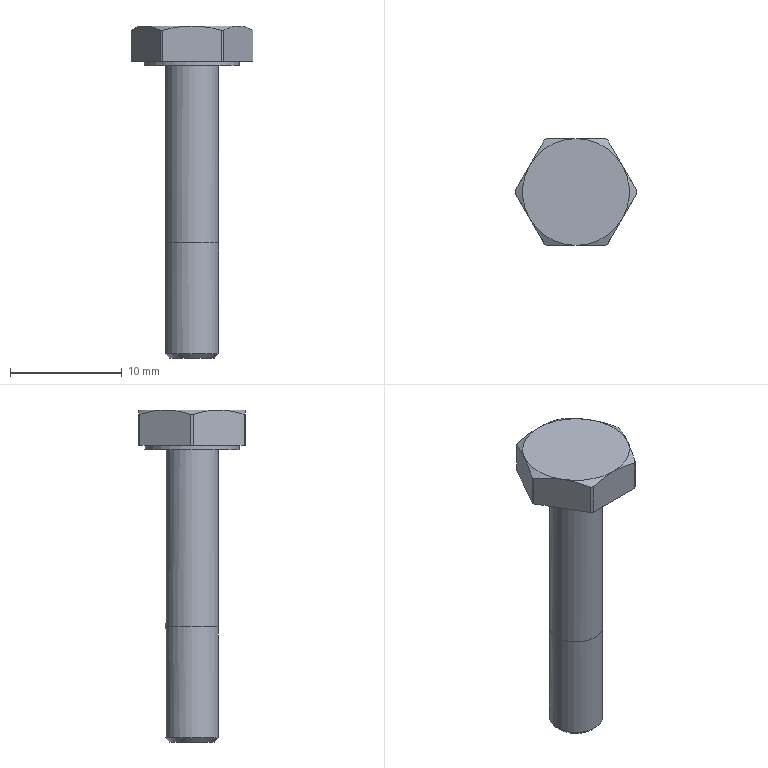Part | NX | features solid 2 | 1 solid | 26 faces | box 10.922 x 9.576 x 29.775 mm | volume 739.727 mm3 | plane 10 | cylinder 9 | cone 7 | commonest cylinder face diameters 10.922 x6 4.763 x2 8.509 x1
STEP:
#1=CARTESIAN_POINT('',(-2.381,0.,-3.581));
#2=VERTEX_POINT('',#1);
#3=CARTESIAN_POINT('',(0.,0.,-3.581));
#4=DIRECTION('',(0.,0.,-1.));
#5=DIRECTION('',(-1.,0.,0.));
#6=AXIS2_PLACEMENT_3D('',#3,#4,#5);
#7=CIRCLE('',#6,2.381);
#8=EDGE_CURVE('',#2,#2,#7,.T.);
#9=ORIENTED_EDGE('',*,*,#8,.T.);
#10=EDGE_LOOP('',(#9));
#11=FACE_BOUND('',#10,.T.);
#12=CARTESIAN_POINT('',(-2.381,0.,-19.456));
#13=VERTEX_POINT('',#12);
#14=CARTESIAN_POINT('',(-1.866,1.866,-19.456));
#15=CARTESIAN_POINT('',(-2.639,0.,-19.456));
#16=CARTESIAN_POINT('',(-1.866,-1.866,-19.456));
#17=CARTESIAN_POINT('',(0.,-2.639,-19.456));
#18=CARTESIAN_POINT('',(1.866,-1.866,-19.456));
#19=CARTESIAN_POINT('',(2.639,0.,-19.456));
#20=CARTESIAN_POINT('',(1.866,1.866,-19.456));
#21=CARTESIAN_POINT('',(0.,2.639,-19.456));
#22=CARTESIAN_POINT('',(-1.866,1.866,-19.456));
#23=CARTESIAN_POINT('',(-2.639,0.,-19.456));
#24=CARTESIAN_POINT('',(-1.866,-1.866,-19.456));
#25=B_SPLINE_CURVE_WITH_KNOTS('',3,(#14,#15,#16,#17,#18,#19,#20,#21,#22,#23,#24),.UNSPECIFIED.,.T.,.F.,(1,1,1,1,1,1,1,1,1,1,1,1,1,1,1),(-0.375,-0.25,-0.125,0.,0.125,0.25,0.375,0.5,0.625,0.75,0.875,1.,1.125,1.25,1.375),.UNSPECIFIED.);
#26=EDGE_CURVE('',#13,#13,#25,.T.);
#27=ORIENTED_EDGE('',*,*,#26,.T.);
#28=EDGE_LOOP('',(#27));
#29=FACE_BOUND('',#28,.T.);
#30=CARTESIAN_POINT('',(0.,0.,0.));
#31=DIRECTION('',(0.,0.,-1.));
#32=DIRECTION('',(-1.,0.,0.));
#33=AXIS2_PLACEMENT_3D('',#30,#31,#32);
#34=CYLINDRICAL_SURFACE('',#33,2.381);
#35=ADVANCED_FACE('',(#11,#29),#34,.T.);
#36=CARTESIAN_POINT('',(2.627,4.788,-3.175));
#37=VERTEX_POINT('',#36);
#38=CARTESIAN_POINT('',(2.833,4.669,-3.175));
#39=VERTEX_POINT('',#38);
#40=CARTESIAN_POINT('',(0.,0.,-3.175));
#41=DIRECTION('',(0.,0.,-1.));
#42=DIRECTION('',(-1.,0.,0.));
#43=AXIS2_PLACEMENT_3D('',#40,#41,#42);
#44=CIRCLE('',#43,5.461);
#45=EDGE_CURVE('',#37,#39,#44,.T.);
#46=ORIENTED_EDGE('',*,*,#45,.F.);
#47=CARTESIAN_POINT('',(2.627,4.788,-0.3886));
#48=VERTEX_POINT('',#47);
#49=CARTESIAN_POINT('',(2.627,4.788,0.));
#50=DIRECTION('',(0.,0.,-1.));
#51=VECTOR('',#50,1000.);
#52=LINE('',#49,#51);
#53=EDGE_CURVE('',#37,#48,#52,.F.);
#54=ORIENTED_EDGE('',*,*,#53,.T.);
#55=CARTESIAN_POINT('',(2.833,4.669,-0.3886));
#56=VERTEX_POINT('',#55);
#57=CARTESIAN_POINT('',(0.,0.,-0.3886));
#58=DIRECTION('',(0.,0.,-1.));
#59=DIRECTION('',(-1.,0.,0.));
#60=AXIS2_PLACEMENT_3D('',#57,#58,#59);
#61=CIRCLE('',#60,5.461);
#62=EDGE_CURVE('',#48,#56,#61,.T.);
#63=ORIENTED_EDGE('',*,*,#62,.T.);
#64=CARTESIAN_POINT('',(2.833,4.669,0.));
#65=DIRECTION('',(0.,0.,-1.));
#66=VECTOR('',#65,1000.);
#67=LINE('',#64,#66);
#68=EDGE_CURVE('',#56,#39,#67,.T.);
#69=ORIENTED_EDGE('',*,*,#68,.T.);
#70=EDGE_LOOP('',(#46,#54,#63,#69));
#71=FACE_BOUND('',#70,.T.);
#72=CARTESIAN_POINT('',(0.,0.,0.));
#73=DIRECTION('',(0.,0.,-1.));
#74=DIRECTION('',(-1.,0.,0.));
#75=AXIS2_PLACEMENT_3D('',#72,#73,#74);
#76=CYLINDRICAL_SURFACE('',#75,5.461);
#77=ADVANCED_FACE('',(#71),#76,.T.);
#78=CARTESIAN_POINT('',(-2.833,4.669,-0.3886));
#79=VERTEX_POINT('',#78);
#80=CARTESIAN_POINT('',(-2.627,4.788,-0.3886));
#81=VERTEX_POINT('',#80);
#82=CARTESIAN_POINT('',(0.,0.,-0.3886));
#83=DIRECTION('',(0.,0.,-1.));
#84=DIRECTION('',(-1.,0.,0.));
#85=AXIS2_PLACEMENT_3D('',#82,#83,#84);
#86=CIRCLE('',#85,5.461);
#87=EDGE_CURVE('',#79,#81,#86,.T.);
#88=ORIENTED_EDGE('',*,*,#87,.T.);
#89=CARTESIAN_POINT('',(-2.627,4.788,-3.175));
#90=VERTEX_POINT('',#89);
#91=CARTESIAN_POINT('',(-2.627,4.788,0.));
#92=DIRECTION('',(0.,0.,-1.));
#93=VECTOR('',#92,1000.);
#94=LINE('',#91,#93);
#95=EDGE_CURVE('',#81,#90,#94,.T.);
#96=ORIENTED_EDGE('',*,*,#95,.T.);
#97=CARTESIAN_POINT('',(-2.833,4.669,-3.175));
#98=VERTEX_POINT('',#97);
#99=CARTESIAN_POINT('',(0.,0.,-3.175));
#100=DIRECTION('',(0.,0.,-1.));
#101=DIRECTION('',(-1.,0.,0.));
#102=AXIS2_PLACEMENT_3D('',#99,#100,#101);
#103=CIRCLE('',#102,5.461);
#104=EDGE_CURVE('',#98,#90,#103,.T.);
#105=ORIENTED_EDGE('',*,*,#104,.F.);
#106=CARTESIAN_POINT('',(-2.833,4.669,0.));
#107=DIRECTION('',(0.,0.,-1.));
#108=VECTOR('',#107,1000.);
#109=LINE('',#106,#108);
#110=EDGE_CURVE('',#98,#79,#109,.F.);
#111=ORIENTED_EDGE('',*,*,#110,.T.);
#112=EDGE_LOOP('',(#88,#96,#105,#111));
#113=FACE_BOUND('',#112,.T.);
#114=CARTESIAN_POINT('',(0.,0.,0.));
#115=DIRECTION('',(0.,0.,-1.));
#116=DIRECTION('',(-1.,0.,0.));
#117=AXIS2_PLACEMENT_3D('',#114,#115,#116);
#118=CYLINDRICAL_SURFACE('',#117,5.461);
#119=ADVANCED_FACE('',(#113),#118,.T.);
#120=CARTESIAN_POINT('',(-5.46,-0.1193,-0.3886));
#121=VERTEX_POINT('',#120);
#122=CARTESIAN_POINT('',(-5.46,0.1193,-0.3886));
#123=VERTEX_POINT('',#122);
#124=CARTESIAN_POINT('',(0.,0.,-0.3886));
#125=DIRECTION('',(0.,0.,-1.));
#126=DIRECTION('',(-1.,0.,0.));
#127=AXIS2_PLACEMENT_3D('',#124,#125,#126);
#128=CIRCLE('',#127,5.461);
#129=EDGE_CURVE('',#121,#123,#128,.T.);
#130=ORIENTED_EDGE('',*,*,#129,.T.);
#131=CARTESIAN_POINT('',(-5.46,0.1193,-3.175));
#132=VERTEX_POINT('',#131);
#133=CARTESIAN_POINT('',(-5.46,0.1193,0.));
#134=DIRECTION('',(0.,0.,-1.));
#135=VECTOR('',#134,1000.);
#136=LINE('',#133,#135);
#137=EDGE_CURVE('',#123,#132,#136,.T.);
#138=ORIENTED_EDGE('',*,*,#137,.T.);
#139=CARTESIAN_POINT('',(-5.46,-0.1193,-3.175));
#140=VERTEX_POINT('',#139);
#141=CARTESIAN_POINT('',(0.,0.,-3.175));
#142=DIRECTION('',(0.,0.,-1.));
#143=DIRECTION('',(-1.,0.,0.));
#144=AXIS2_PLACEMENT_3D('',#141,#142,#143);
#145=CIRCLE('',#144,5.461);
#146=EDGE_CURVE('',#140,#132,#145,.T.);
#147=ORIENTED_EDGE('',*,*,#146,.F.);
#148=CARTESIAN_POINT('',(-5.46,-0.1193,0.));
#149=DIRECTION('',(0.,0.,-1.));
#150=VECTOR('',#149,1000.);
#151=LINE('',#148,#150);
#152=EDGE_CURVE('',#140,#121,#151,.F.);
#153=ORIENTED_EDGE('',*,*,#152,.T.);
#154=EDGE_LOOP('',(#130,#138,#147,#153));
#155=FACE_BOUND('',#154,.T.);
#156=CARTESIAN_POINT('',(0.,0.,0.));
#157=DIRECTION('',(0.,0.,-1.));
#158=DIRECTION('',(-1.,0.,0.));
#159=AXIS2_PLACEMENT_3D('',#156,#157,#158);
#160=CYLINDRICAL_SURFACE('',#159,5.461);
#161=ADVANCED_FACE('',(#155),#160,.T.);
#162=CARTESIAN_POINT('',(-2.627,-4.788,-0.3886));
#163=VERTEX_POINT('',#162);
#164=CARTESIAN_POINT('',(-2.833,-4.669,-0.3886));
#165=VERTEX_POINT('',#164);
#166=CARTESIAN_POINT('',(0.,0.,-0.3886));
#167=DIRECTION('',(0.,0.,-1.));
#168=DIRECTION('',(-1.,0.,0.));
#169=AXIS2_PLACEMENT_3D('',#166,#167,#168);
#170=CIRCLE('',#169,5.461);
#171=EDGE_CURVE('',#163,#165,#170,.T.);
#172=ORIENTED_EDGE('',*,*,#171,.T.);
#173=CARTESIAN_POINT('',(-2.833,-4.669,-3.175));
#174=VERTEX_POINT('',#173);
#175=CARTESIAN_POINT('',(-2.833,-4.669,0.));
#176=DIRECTION('',(0.,0.,-1.));
#177=VECTOR('',#176,1000.);
#178=LINE('',#175,#177);
#179=EDGE_CURVE('',#165,#174,#178,.T.);
#180=ORIENTED_EDGE('',*,*,#179,.T.);
#181=CARTESIAN_POINT('',(-2.627,-4.788,-3.175));
#182=VERTEX_POINT('',#181);
#183=CARTESIAN_POINT('',(0.,0.,-3.175));
#184=DIRECTION('',(0.,0.,-1.));
#185=DIRECTION('',(-1.,0.,0.));
#186=AXIS2_PLACEMENT_3D('',#183,#184,#185);
#187=CIRCLE('',#186,5.461);
#188=EDGE_CURVE('',#182,#174,#187,.T.);
#189=ORIENTED_EDGE('',*,*,#188,.F.);
#190=CARTESIAN_POINT('',(-2.627,-4.788,0.));
#191=DIRECTION('',(0.,0.,-1.));
#192=VECTOR('',#191,1000.);
#193=LINE('',#190,#192);
#194=EDGE_CURVE('',#182,#163,#193,.F.);
#195=ORIENTED_EDGE('',*,*,#194,.T.);
#196=EDGE_LOOP('',(#172,#180,#189,#195));
#197=FACE_BOUND('',#196,.T.);
#198=CARTESIAN_POINT('',(0.,0.,0.));
#199=DIRECTION('',(0.,0.,-1.));
#200=DIRECTION('',(-1.,0.,0.));
#201=AXIS2_PLACEMENT_3D('',#198,#199,#200);
#202=CYLINDRICAL_SURFACE('',#201,5.461);
#203=ADVANCED_FACE('',(#197),#202,.T.);
#204=CARTESIAN_POINT('',(2.833,-4.669,-0.3886));
#205=VERTEX_POINT('',#204);
#206=CARTESIAN_POINT('',(2.627,-4.788,-0.3886));
#207=VERTEX_POINT('',#206);
#208=CARTESIAN_POINT('',(0.,0.,-0.3886));
#209=DIRECTION('',(0.,0.,-1.));
#210=DIRECTION('',(-1.,0.,0.));
#211=AXIS2_PLACEMENT_3D('',#208,#209,#210);
#212=CIRCLE('',#211,5.461);
#213=EDGE_CURVE('',#205,#207,#212,.T.);
#214=ORIENTED_EDGE('',*,*,#213,.T.);
#215=CARTESIAN_POINT('',(2.627,-4.788,-3.175));
#216=VERTEX_POINT('',#215);
#217=CARTESIAN_POINT('',(2.627,-4.788,0.));
#218=DIRECTION('',(0.,0.,-1.));
#219=VECTOR('',#218,1000.);
#220=LINE('',#217,#219);
#221=EDGE_CURVE('',#207,#216,#220,.T.);
#222=ORIENTED_EDGE('',*,*,#221,.T.);
#223=CARTESIAN_POINT('',(2.833,-4.669,-3.175));
#224=VERTEX_POINT('',#223);
#225=CARTESIAN_POINT('',(0.,0.,-3.175));
#226=DIRECTION('',(0.,0.,-1.));
#227=DIRECTION('',(-1.,0.,0.));
#228=AXIS2_PLACEMENT_3D('',#225,#226,#227);
#229=CIRCLE('',#228,5.461);
#230=EDGE_CURVE('',#224,#216,#229,.T.);
#231=ORIENTED_EDGE('',*,*,#230,.F.);
#232=CARTESIAN_POINT('',(2.833,-4.669,0.));
#233=DIRECTION('',(0.,0.,-1.));
#234=VECTOR('',#233,1000.);
#235=LINE('',#232,#234);
#236=EDGE_CURVE('',#224,#205,#235,.F.);
#237=ORIENTED_EDGE('',*,*,#236,.T.);
#238=EDGE_LOOP('',(#214,#222,#231,#237));
#239=FACE_BOUND('',#238,.T.);
#240=CARTESIAN_POINT('',(0.,0.,0.));
#241=DIRECTION('',(0.,0.,-1.));
#242=DIRECTION('',(-1.,0.,0.));
#243=AXIS2_PLACEMENT_3D('',#240,#241,#242);
#244=CYLINDRICAL_SURFACE('',#243,5.461);
#245=ADVANCED_FACE('',(#239),#244,.T.);
#246=ORIENTED_EDGE('',*,*,#62,.F.);
#247=CARTESIAN_POINT('',(0.,4.788,0.));
#248=VERTEX_POINT('',#247);
#249=CARTESIAN_POINT('',(0.,4.788,0.));
#250=CARTESIAN_POINT('',(0.8868,4.788,0.));
#251=CARTESIAN_POINT('',(1.776,4.788,-0.1525));
#252=CARTESIAN_POINT('',(2.627,4.788,-0.3886));
#253=B_SPLINE_CURVE_WITH_KNOTS('',3,(#249,#250,#251,#252),.UNSPECIFIED.,.F.,.F.,(4,4),(0.007722,0.01038),.UNSPECIFIED.);
#254=EDGE_CURVE('',#48,#248,#253,.F.);
#255=ORIENTED_EDGE('',*,*,#254,.T.);
#256=CARTESIAN_POINT('',(4.146,2.394,0.));
#257=VERTEX_POINT('',#256);
#258=CARTESIAN_POINT('',(0.,0.,0.));
#259=DIRECTION('',(0.,0.,-1.));
#260=DIRECTION('',(-1.,0.,0.));
#261=AXIS2_PLACEMENT_3D('',#258,#259,#260);
#262=CIRCLE('',#261,4.788);
#263=EDGE_CURVE('',#248,#257,#262,.T.);
#264=ORIENTED_EDGE('',*,*,#263,.T.);
#265=CARTESIAN_POINT('',(4.146,2.394,0.));
#266=CARTESIAN_POINT('',(3.703,3.163,0.));
#267=CARTESIAN_POINT('',(3.262,3.925,-0.1503));
#268=CARTESIAN_POINT('',(2.833,4.669,-0.3886));
#269=B_SPLINE_CURVE_WITH_KNOTS('',3,(#265,#266,#267,#268),.UNSPECIFIED.,.F.,.F.,(4,4),(0.002655,0.005296),.UNSPECIFIED.);
#270=EDGE_CURVE('',#257,#56,#269,.T.);
#271=ORIENTED_EDGE('',*,*,#270,.T.);
#272=EDGE_LOOP('',(#246,#255,#264,#271));
#273=FACE_BOUND('',#272,.T.);
#274=CARTESIAN_POINT('',(0.,0.,-0.3886));
#275=DIRECTION('',(0.,0.,-1.));
#276=DIRECTION('',(-1.,0.,0.));
#277=AXIS2_PLACEMENT_3D('',#274,#275,#276);
#278=CONICAL_SURFACE('',#277,5.461,1.047);
#279=ADVANCED_FACE('',(#273),#278,.T.);
#280=CARTESIAN_POINT('',(-4.146,2.394,0.));
#281=VERTEX_POINT('',#280);
#282=CARTESIAN_POINT('',(0.,0.,0.));
#283=DIRECTION('',(0.,0.,-1.));
#284=DIRECTION('',(-1.,0.,0.));
#285=AXIS2_PLACEMENT_3D('',#282,#283,#284);
#286=CIRCLE('',#285,4.788);
#287=EDGE_CURVE('',#281,#248,#286,.T.);
#288=ORIENTED_EDGE('',*,*,#287,.T.);
#289=CARTESIAN_POINT('',(-2.627,4.788,-0.3886));
#290=CARTESIAN_POINT('',(-1.77,4.788,-0.1508));
#291=CARTESIAN_POINT('',(-0.8866,4.788,0.));
#292=CARTESIAN_POINT('',(0.,4.788,0.));
#293=B_SPLINE_CURVE_WITH_KNOTS('',3,(#289,#290,#291,#292),.UNSPECIFIED.,.F.,.F.,(4,4),(0.005068,0.007722),.UNSPECIFIED.);
#294=EDGE_CURVE('',#248,#81,#293,.F.);
#295=ORIENTED_EDGE('',*,*,#294,.T.);
#296=ORIENTED_EDGE('',*,*,#87,.F.);
#297=CARTESIAN_POINT('',(-2.833,4.669,-0.3886));
#298=CARTESIAN_POINT('',(-3.264,3.923,-0.1495));
#299=CARTESIAN_POINT('',(-3.7,3.167,0.));
#300=CARTESIAN_POINT('',(-4.146,2.394,0.));
#301=B_SPLINE_CURVE_WITH_KNOTS('',3,(#297,#298,#299,#300),.UNSPECIFIED.,.F.,.F.,(4,4),(0.00000074,0.002655),.UNSPECIFIED.);
#302=EDGE_CURVE('',#79,#281,#301,.T.);
#303=ORIENTED_EDGE('',*,*,#302,.T.);
#304=EDGE_LOOP('',(#288,#295,#296,#303));
#305=FACE_BOUND('',#304,.T.);
#306=CARTESIAN_POINT('',(0.,0.,-0.3886));
#307=DIRECTION('',(0.,0.,-1.));
#308=DIRECTION('',(-1.,0.,0.));
#309=AXIS2_PLACEMENT_3D('',#306,#307,#308);
#310=CONICAL_SURFACE('',#309,5.461,1.047);
#311=ADVANCED_FACE('',(#305),#310,.T.);
#312=CARTESIAN_POINT('',(-4.146,-2.394,0.));
#313=VERTEX_POINT('',#312);
#314=CARTESIAN_POINT('',(0.,0.,0.));
#315=DIRECTION('',(0.,0.,-1.));
#316=DIRECTION('',(-1.,0.,0.));
#317=AXIS2_PLACEMENT_3D('',#314,#315,#316);
#318=CIRCLE('',#317,4.788);
#319=EDGE_CURVE('',#313,#281,#318,.T.);
#320=ORIENTED_EDGE('',*,*,#319,.T.);
#321=CARTESIAN_POINT('',(-4.146,2.394,0.));
#322=CARTESIAN_POINT('',(-4.59,1.625,0.));
#323=CARTESIAN_POINT('',(-5.031,0.8625,-0.1503));
#324=CARTESIAN_POINT('',(-5.46,0.1193,-0.3886));
#325=B_SPLINE_CURVE_WITH_KNOTS('',3,(#321,#322,#323,#324),.UNSPECIFIED.,.F.,.F.,(4,4),(0.002655,0.005296),.UNSPECIFIED.);
#326=EDGE_CURVE('',#281,#123,#325,.T.);
#327=ORIENTED_EDGE('',*,*,#326,.T.);
#328=ORIENTED_EDGE('',*,*,#129,.F.);
#329=CARTESIAN_POINT('',(-5.46,-0.1193,-0.3886));
#330=CARTESIAN_POINT('',(-5.029,-0.8651,-0.1495));
#331=CARTESIAN_POINT('',(-4.593,-1.621,0.));
#332=CARTESIAN_POINT('',(-4.146,-2.394,0.));
#333=B_SPLINE_CURVE_WITH_KNOTS('',3,(#329,#330,#331,#332),.UNSPECIFIED.,.F.,.F.,(4,4),(0.00000074,0.002655),.UNSPECIFIED.);
#334=EDGE_CURVE('',#121,#313,#333,.T.);
#335=ORIENTED_EDGE('',*,*,#334,.T.);
#336=EDGE_LOOP('',(#320,#327,#328,#335));
#337=FACE_BOUND('',#336,.T.);
#338=CARTESIAN_POINT('',(0.,0.,-0.3886));
#339=DIRECTION('',(0.,0.,-1.));
#340=DIRECTION('',(-1.,0.,0.));
#341=AXIS2_PLACEMENT_3D('',#338,#339,#340);
#342=CONICAL_SURFACE('',#341,5.461,1.047);
#343=ADVANCED_FACE('',(#337),#342,.T.);
#344=CARTESIAN_POINT('',(0.,-4.788,0.));
#345=VERTEX_POINT('',#344);
#346=CARTESIAN_POINT('',(0.,0.,0.));
#347=DIRECTION('',(0.,0.,-1.));
#348=DIRECTION('',(-1.,0.,0.));
#349=AXIS2_PLACEMENT_3D('',#346,#347,#348);
#350=CIRCLE('',#349,4.788);
#351=EDGE_CURVE('',#345,#313,#350,.T.);
#352=ORIENTED_EDGE('',*,*,#351,.T.);
#353=CARTESIAN_POINT('',(-4.146,-2.394,0.));
#354=CARTESIAN_POINT('',(-3.703,-3.163,0.));
#355=CARTESIAN_POINT('',(-3.262,-3.925,-0.1503));
#356=CARTESIAN_POINT('',(-2.833,-4.669,-0.3886));
#357=B_SPLINE_CURVE_WITH_KNOTS('',3,(#353,#354,#355,#356),.UNSPECIFIED.,.F.,.F.,(4,4),(0.002655,0.005296),.UNSPECIFIED.);
#358=EDGE_CURVE('',#313,#165,#357,.T.);
#359=ORIENTED_EDGE('',*,*,#358,.T.);
#360=ORIENTED_EDGE('',*,*,#171,.F.);
#361=CARTESIAN_POINT('',(-2.627,-4.788,-0.3886));
#362=CARTESIAN_POINT('',(-1.77,-4.788,-0.1508));
#363=CARTESIAN_POINT('',(-0.8866,-4.788,0.));
#364=CARTESIAN_POINT('',(0.,-4.788,0.));
#365=B_SPLINE_CURVE_WITH_KNOTS('',3,(#361,#362,#363,#364),.UNSPECIFIED.,.F.,.F.,(4,4),(0.005068,0.007722),.UNSPECIFIED.);
#366=EDGE_CURVE('',#163,#345,#365,.T.);
#367=ORIENTED_EDGE('',*,*,#366,.T.);
#368=EDGE_LOOP('',(#352,#359,#360,#367));
#369=FACE_BOUND('',#368,.T.);
#370=CARTESIAN_POINT('',(0.,0.,-0.3886));
#371=DIRECTION('',(0.,0.,-1.));
#372=DIRECTION('',(-1.,0.,0.));
#373=AXIS2_PLACEMENT_3D('',#370,#371,#372);
#374=CONICAL_SURFACE('',#373,5.461,1.047);
#375=ADVANCED_FACE('',(#369),#374,.T.);
#376=CARTESIAN_POINT('',(4.146,-2.394,0.));
#377=VERTEX_POINT('',#376);
#378=CARTESIAN_POINT('',(0.,0.,0.));
#379=DIRECTION('',(0.,0.,-1.));
#380=DIRECTION('',(-1.,0.,0.));
#381=AXIS2_PLACEMENT_3D('',#378,#379,#380);
#382=CIRCLE('',#381,4.788);
#383=EDGE_CURVE('',#377,#345,#382,.T.);
#384=ORIENTED_EDGE('',*,*,#383,.T.);
#385=CARTESIAN_POINT('',(0.,-4.788,0.));
#386=CARTESIAN_POINT('',(0.8868,-4.788,0.));
#387=CARTESIAN_POINT('',(1.776,-4.788,-0.1525));
#388=CARTESIAN_POINT('',(2.627,-4.788,-0.3886));
#389=B_SPLINE_CURVE_WITH_KNOTS('',3,(#385,#386,#387,#388),.UNSPECIFIED.,.F.,.F.,(4,4),(0.007722,0.01038),.UNSPECIFIED.);
#390=EDGE_CURVE('',#345,#207,#389,.T.);
#391=ORIENTED_EDGE('',*,*,#390,.T.);
#392=ORIENTED_EDGE('',*,*,#213,.F.);
#393=CARTESIAN_POINT('',(2.833,-4.669,-0.3886));
#394=CARTESIAN_POINT('',(3.264,-3.923,-0.1495));
#395=CARTESIAN_POINT('',(3.7,-3.167,0.));
#396=CARTESIAN_POINT('',(4.146,-2.394,0.));
#397=B_SPLINE_CURVE_WITH_KNOTS('',3,(#393,#394,#395,#396),.UNSPECIFIED.,.F.,.F.,(4,4),(0.00000074,0.002655),.UNSPECIFIED.);
#398=EDGE_CURVE('',#205,#377,#397,.T.);
#399=ORIENTED_EDGE('',*,*,#398,.T.);
#400=EDGE_LOOP('',(#384,#391,#392,#399));
#401=FACE_BOUND('',#400,.T.);
#402=CARTESIAN_POINT('',(0.,0.,-0.3886));
#403=DIRECTION('',(0.,0.,-1.));
#404=DIRECTION('',(-1.,0.,0.));
#405=AXIS2_PLACEMENT_3D('',#402,#403,#404);
#406=CONICAL_SURFACE('',#405,5.461,1.047);
#407=ADVANCED_FACE('',(#401),#406,.T.);
#408=ORIENTED_EDGE('',*,*,#104,.T.);
#409=CARTESIAN_POINT('',(4.255,4.788,-3.175));
#410=DIRECTION('',(1.,0.,0.));
#411=VECTOR('',#410,1000.);
#412=LINE('',#409,#411);
#413=EDGE_CURVE('',#90,#37,#412,.T.);
#414=ORIENTED_EDGE('',*,*,#413,.T.);
#415=ORIENTED_EDGE('',*,*,#45,.T.);
#416=CARTESIAN_POINT('',(5.46,0.1193,-3.175));
#417=VERTEX_POINT('',#416);
#418=CARTESIAN_POINT('',(5.21,0.5517,-3.175));
#419=DIRECTION('',(0.5,-0.866,0.));
#420=VECTOR('',#419,1000.);
#421=LINE('',#418,#420);
#422=EDGE_CURVE('',#39,#417,#421,.T.);
#423=ORIENTED_EDGE('',*,*,#422,.T.);
#424=CARTESIAN_POINT('',(5.46,-0.1193,-3.175));
#425=VERTEX_POINT('',#424);
#426=CARTESIAN_POINT('',(0.,0.,-3.175));
#427=DIRECTION('',(0.,0.,-1.));
#428=DIRECTION('',(-1.,0.,0.));
#429=AXIS2_PLACEMENT_3D('',#426,#427,#428);
#430=CIRCLE('',#429,5.461);
#431=EDGE_CURVE('',#417,#425,#430,.T.);
#432=ORIENTED_EDGE('',*,*,#431,.T.);
#433=CARTESIAN_POINT('',(5.21,-0.5517,-3.175));
#434=DIRECTION('',(-0.5,-0.866,0.));
#435=VECTOR('',#434,1000.);
#436=LINE('',#433,#435);
#437=EDGE_CURVE('',#425,#224,#436,.T.);
#438=ORIENTED_EDGE('',*,*,#437,.T.);
#439=ORIENTED_EDGE('',*,*,#230,.T.);
#440=CARTESIAN_POINT('',(4.255,-4.788,-3.175));
#441=DIRECTION('',(-1.,0.,0.));
#442=VECTOR('',#441,1000.);
#443=LINE('',#440,#442);
#444=EDGE_CURVE('',#216,#182,#443,.T.);
#445=ORIENTED_EDGE('',*,*,#444,.T.);
#446=ORIENTED_EDGE('',*,*,#188,.T.);
#447=CARTESIAN_POINT('',(-3.083,-4.236,-3.175));
#448=DIRECTION('',(-0.5,0.866,0.));
#449=VECTOR('',#448,1000.);
#450=LINE('',#447,#449);
#451=EDGE_CURVE('',#174,#140,#450,.T.);
#452=ORIENTED_EDGE('',*,*,#451,.T.);
#453=ORIENTED_EDGE('',*,*,#146,.T.);
#454=CARTESIAN_POINT('',(-3.083,4.236,-3.175));
#455=DIRECTION('',(0.5,0.866,0.));
#456=VECTOR('',#455,1000.);
#457=LINE('',#454,#456);
#458=EDGE_CURVE('',#132,#98,#457,.T.);
#459=ORIENTED_EDGE('',*,*,#458,.T.);
#460=EDGE_LOOP('',(#408,#414,#415,#423,#432,#438,#439,#445,#446,#452,#453,#459));
#461=FACE_BOUND('',#460,.T.);
#462=CARTESIAN_POINT('',(-4.255,0.,-3.175));
#463=VERTEX_POINT('',#462);
#464=CARTESIAN_POINT('',(0.,0.,-3.175));
#465=DIRECTION('',(0.,0.,-1.));
#466=DIRECTION('',(-1.,0.,0.));
#467=AXIS2_PLACEMENT_3D('',#464,#465,#466);
#468=CIRCLE('',#467,4.255);
#469=EDGE_CURVE('',#463,#463,#468,.T.);
#470=ORIENTED_EDGE('',*,*,#469,.F.);
#471=EDGE_LOOP('',(#470));
#472=FACE_BOUND('',#471,.T.);
#473=CARTESIAN_POINT('',(4.255,0.,-3.175));
#474=DIRECTION('',(0.,0.,-1.));
#475=DIRECTION('',(-1.,0.,0.));
#476=AXIS2_PLACEMENT_3D('',#473,#474,#475);
#477=PLANE('',#476);
#478=ADVANCED_FACE('',(#461,#472),#477,.T.);
#479=CARTESIAN_POINT('',(5.46,0.1193,-0.3886));
#480=VERTEX_POINT('',#479);
#481=CARTESIAN_POINT('',(5.46,-0.1193,-0.3886));
#482=VERTEX_POINT('',#481);
#483=CARTESIAN_POINT('',(0.,0.,-0.3886));
#484=DIRECTION('',(0.,0.,-1.));
#485=DIRECTION('',(-1.,0.,0.));
#486=AXIS2_PLACEMENT_3D('',#483,#484,#485);
#487=CIRCLE('',#486,5.461);
#488=EDGE_CURVE('',#480,#482,#487,.T.);
#489=ORIENTED_EDGE('',*,*,#488,.T.);
#490=CARTESIAN_POINT('',(5.46,-0.1193,0.));
#491=DIRECTION('',(0.,0.,-1.));
#492=VECTOR('',#491,1000.);
#493=LINE('',#490,#492);
#494=EDGE_CURVE('',#482,#425,#493,.T.);
#495=ORIENTED_EDGE('',*,*,#494,.T.);
#496=ORIENTED_EDGE('',*,*,#431,.F.);
#497=CARTESIAN_POINT('',(5.46,0.1193,0.));
#498=DIRECTION('',(0.,0.,-1.));
#499=VECTOR('',#498,1000.);
#500=LINE('',#497,#499);
#501=EDGE_CURVE('',#417,#480,#500,.F.);
#502=ORIENTED_EDGE('',*,*,#501,.T.);
#503=EDGE_LOOP('',(#489,#495,#496,#502));
#504=FACE_BOUND('',#503,.T.);
#505=CARTESIAN_POINT('',(0.,0.,0.));
#506=DIRECTION('',(0.,0.,-1.));
#507=DIRECTION('',(-1.,0.,0.));
#508=AXIS2_PLACEMENT_3D('',#505,#506,#507);
#509=CYLINDRICAL_SURFACE('',#508,5.461);
#510=ADVANCED_FACE('',(#504),#509,.T.);
#511=CARTESIAN_POINT('',(0.,0.,0.));
#512=DIRECTION('',(0.,0.,-1.));
#513=DIRECTION('',(-1.,0.,0.));
#514=AXIS2_PLACEMENT_3D('',#511,#512,#513);
#515=CIRCLE('',#514,4.788);
#516=EDGE_CURVE('',#257,#377,#515,.T.);
#517=ORIENTED_EDGE('',*,*,#516,.T.);
#518=CARTESIAN_POINT('',(4.146,-2.394,0.));
#519=CARTESIAN_POINT('',(4.59,-1.625,0.));
#520=CARTESIAN_POINT('',(5.031,-0.8625,-0.1503));
#521=CARTESIAN_POINT('',(5.46,-0.1193,-0.3886));
#522=B_SPLINE_CURVE_WITH_KNOTS('',3,(#518,#519,#520,#521),.UNSPECIFIED.,.F.,.F.,(4,4),(0.002655,0.005296),.UNSPECIFIED.);
#523=EDGE_CURVE('',#377,#482,#522,.T.);
#524=ORIENTED_EDGE('',*,*,#523,.T.);
#525=ORIENTED_EDGE('',*,*,#488,.F.);
#526=CARTESIAN_POINT('',(5.46,0.1193,-0.3886));
#527=CARTESIAN_POINT('',(5.029,0.8651,-0.1495));
#528=CARTESIAN_POINT('',(4.593,1.621,0.));
#529=CARTESIAN_POINT('',(4.146,2.394,0.));
#530=B_SPLINE_CURVE_WITH_KNOTS('',3,(#526,#527,#528,#529),.UNSPECIFIED.,.F.,.F.,(4,4),(0.00000074,0.002655),.UNSPECIFIED.);
#531=EDGE_CURVE('',#480,#257,#530,.T.);
#532=ORIENTED_EDGE('',*,*,#531,.T.);
#533=EDGE_LOOP('',(#517,#524,#525,#532));
#534=FACE_BOUND('',#533,.T.);
#535=CARTESIAN_POINT('',(0.,0.,-0.3886));
#536=DIRECTION('',(0.,0.,-1.));
#537=DIRECTION('',(-1.,0.,0.));
#538=AXIS2_PLACEMENT_3D('',#535,#536,#537);
#539=CONICAL_SURFACE('',#538,5.461,1.047);
#540=ADVANCED_FACE('',(#534),#539,.T.);
#541=ORIENTED_EDGE('',*,*,#287,.F.);
#542=ORIENTED_EDGE('',*,*,#319,.F.);
#543=ORIENTED_EDGE('',*,*,#351,.F.);
#544=ORIENTED_EDGE('',*,*,#383,.F.);
#545=ORIENTED_EDGE('',*,*,#516,.F.);
#546=ORIENTED_EDGE('',*,*,#263,.F.);
#547=EDGE_LOOP('',(#541,#542,#543,#544,#545,#546));
#548=FACE_BOUND('',#547,.T.);
#549=CARTESIAN_POINT('',(4.788,0.,0.));
#550=DIRECTION('',(0.,0.,1.));
#551=DIRECTION('',(1.,0.,0.));
#552=AXIS2_PLACEMENT_3D('',#549,#550,#551);
#553=PLANE('',#552);
#554=ADVANCED_FACE('',(#548),#553,.T.);
#555=CARTESIAN_POINT('',(-2.,0.,-29.775));
#556=VERTEX_POINT('',#555);
#557=CARTESIAN_POINT('',(0.,0.,-29.775));
#558=DIRECTION('',(0.,0.,-1.));
#559=DIRECTION('',(-1.,0.,0.));
#560=AXIS2_PLACEMENT_3D('',#557,#558,#559);
#561=CIRCLE('',#560,2.);
#562=EDGE_CURVE('',#556,#556,#561,.T.);
#563=ORIENTED_EDGE('',*,*,#562,.T.);
#564=EDGE_LOOP('',(#563));
#565=FACE_BOUND('',#564,.T.);
#566=CARTESIAN_POINT('',(0.,0.,-29.775));
#567=DIRECTION('',(0.,0.,-1.));
#568=DIRECTION('',(-1.,0.,0.));
#569=AXIS2_PLACEMENT_3D('',#566,#567,#568);
#570=PLANE('',#569);
#571=ADVANCED_FACE('',(#565),#570,.T.);
#572=CARTESIAN_POINT('',(-2.381,0.,-29.394));
#573=VERTEX_POINT('',#572);
#574=CARTESIAN_POINT('',(0.,0.,-29.394));
#575=DIRECTION('',(0.,0.,-1.));
#576=DIRECTION('',(-1.,0.,0.));
#577=AXIS2_PLACEMENT_3D('',#574,#575,#576);
#578=CIRCLE('',#577,2.381);
#579=EDGE_CURVE('',#573,#573,#578,.T.);
#580=ORIENTED_EDGE('',*,*,#579,.T.);
#581=EDGE_LOOP('',(#580));
#582=FACE_BOUND('',#581,.T.);
#583=ORIENTED_EDGE('',*,*,#562,.F.);
#584=EDGE_LOOP('',(#583));
#585=FACE_BOUND('',#584,.T.);
#586=CARTESIAN_POINT('',(0.,0.,-29.775));
#587=DIRECTION('',(0.,0.,1.));
#588=DIRECTION('',(1.,0.,0.));
#589=AXIS2_PLACEMENT_3D('',#586,#587,#588);
#590=CONICAL_SURFACE('',#589,2.,0.7854);
#591=ADVANCED_FACE('',(#582,#585),#590,.T.);
#592=ORIENTED_EDGE('',*,*,#26,.F.);
#593=EDGE_LOOP('',(#592));
#594=FACE_BOUND('',#593,.T.);
#595=ORIENTED_EDGE('',*,*,#579,.F.);
#596=EDGE_LOOP('',(#595));
#597=FACE_BOUND('',#596,.T.);
#598=CARTESIAN_POINT('',(0.,0.,0.));
#599=DIRECTION('',(0.,0.,-1.));
#600=DIRECTION('',(-1.,0.,0.));
#601=AXIS2_PLACEMENT_3D('',#598,#599,#600);
#602=CYLINDRICAL_SURFACE('',#601,2.381);
#603=ADVANCED_FACE('',(#594,#597),#602,.T.);
#604=CARTESIAN_POINT('',(-4.255,0.,-3.581));
#605=VERTEX_POINT('',#604);
#606=CARTESIAN_POINT('',(0.,0.,-3.581));
#607=DIRECTION('',(0.,0.,-1.));
#608=DIRECTION('',(-1.,0.,0.));
#609=AXIS2_PLACEMENT_3D('',#606,#607,#608);
#610=CIRCLE('',#609,4.255);
#611=EDGE_CURVE('',#605,#605,#610,.T.);
#612=ORIENTED_EDGE('',*,*,#611,.T.);
#613=EDGE_LOOP('',(#612));
#614=FACE_BOUND('',#613,.T.);
#615=ORIENTED_EDGE('',*,*,#8,.F.);
#616=EDGE_LOOP('',(#615));
#617=FACE_BOUND('',#616,.T.);
#618=CARTESIAN_POINT('',(2.381,0.,-3.581));
#619=DIRECTION('',(0.,0.,-1.));
#620=DIRECTION('',(-1.,0.,0.));
#621=AXIS2_PLACEMENT_3D('',#618,#619,#620);
#622=PLANE('',#621);
#623=ADVANCED_FACE('',(#614,#617),#622,.T.);
#624=ORIENTED_EDGE('',*,*,#469,.T.);
#625=EDGE_LOOP('',(#624));
#626=FACE_BOUND('',#625,.T.);
#627=ORIENTED_EDGE('',*,*,#611,.F.);
#628=EDGE_LOOP('',(#627));
#629=FACE_BOUND('',#628,.T.);
#630=CARTESIAN_POINT('',(0.,0.,0.));
#631=DIRECTION('',(0.,0.,-1.));
#632=DIRECTION('',(-1.,0.,0.));
#633=AXIS2_PLACEMENT_3D('',#630,#631,#632);
#634=CYLINDRICAL_SURFACE('',#633,4.255);
#635=ADVANCED_FACE('',(#626,#629),#634,.T.);
#636=ORIENTED_EDGE('',*,*,#422,.F.);
#637=ORIENTED_EDGE('',*,*,#68,.F.);
#638=ORIENTED_EDGE('',*,*,#270,.F.);
#639=ORIENTED_EDGE('',*,*,#531,.F.);
#640=ORIENTED_EDGE('',*,*,#501,.F.);
#641=EDGE_LOOP('',(#636,#637,#638,#639,#640));
#642=FACE_BOUND('',#641,.T.);
#643=CARTESIAN_POINT('',(5.529,0.,-32.753));
#644=DIRECTION('',(0.866,0.5,0.));
#645=DIRECTION('',(-0.5,0.866,0.));
#646=AXIS2_PLACEMENT_3D('',#643,#644,#645);
#647=PLANE('',#646);
#648=ADVANCED_FACE('',(#642),#647,.T.);
#649=ORIENTED_EDGE('',*,*,#437,.F.);
#650=ORIENTED_EDGE('',*,*,#494,.F.);
#651=ORIENTED_EDGE('',*,*,#523,.F.);
#652=ORIENTED_EDGE('',*,*,#398,.F.);
#653=ORIENTED_EDGE('',*,*,#236,.F.);
#654=EDGE_LOOP('',(#649,#650,#651,#652,#653));
#655=FACE_BOUND('',#654,.T.);
#656=CARTESIAN_POINT('',(2.764,-4.788,-32.753));
#657=DIRECTION('',(0.866,-0.5,0.));
#658=DIRECTION('',(0.5,0.866,0.));
#659=AXIS2_PLACEMENT_3D('',#656,#657,#658);
#660=PLANE('',#659);
#661=ADVANCED_FACE('',(#655),#660,.T.);
#662=ORIENTED_EDGE('',*,*,#444,.F.);
#663=ORIENTED_EDGE('',*,*,#221,.F.);
#664=ORIENTED_EDGE('',*,*,#390,.F.);
#665=ORIENTED_EDGE('',*,*,#366,.F.);
#666=ORIENTED_EDGE('',*,*,#194,.F.);
#667=EDGE_LOOP('',(#662,#663,#664,#665,#666));
#668=FACE_BOUND('',#667,.T.);
#669=CARTESIAN_POINT('',(-2.764,-4.788,-32.753));
#670=DIRECTION('',(0.,-1.,0.));
#671=DIRECTION('',(0.,0.,-1.));
#672=AXIS2_PLACEMENT_3D('',#669,#670,#671);
#673=PLANE('',#672);
#674=ADVANCED_FACE('',(#668),#673,.T.);
#675=ORIENTED_EDGE('',*,*,#451,.F.);
#676=ORIENTED_EDGE('',*,*,#179,.F.);
#677=ORIENTED_EDGE('',*,*,#358,.F.);
#678=ORIENTED_EDGE('',*,*,#334,.F.);
#679=ORIENTED_EDGE('',*,*,#152,.F.);
#680=EDGE_LOOP('',(#675,#676,#677,#678,#679));
#681=FACE_BOUND('',#680,.T.);
#682=CARTESIAN_POINT('',(-5.529,0.,-32.753));
#683=DIRECTION('',(-0.866,-0.5,0.));
#684=DIRECTION('',(0.5,-0.866,0.));
#685=AXIS2_PLACEMENT_3D('',#682,#683,#684);
#686=PLANE('',#685);
#687=ADVANCED_FACE('',(#681),#686,.T.);
#688=ORIENTED_EDGE('',*,*,#458,.F.);
#689=ORIENTED_EDGE('',*,*,#137,.F.);
#690=ORIENTED_EDGE('',*,*,#326,.F.);
#691=ORIENTED_EDGE('',*,*,#302,.F.);
#692=ORIENTED_EDGE('',*,*,#110,.F.);
#693=EDGE_LOOP('',(#688,#689,#690,#691,#692));
#694=FACE_BOUND('',#693,.T.);
#695=CARTESIAN_POINT('',(-2.764,4.788,-32.753));
#696=DIRECTION('',(-0.866,0.5,0.));
#697=DIRECTION('',(-0.5,-0.866,0.));
#698=AXIS2_PLACEMENT_3D('',#695,#696,#697);
#699=PLANE('',#698);
#700=ADVANCED_FACE('',(#694),#699,.T.);
#701=ORIENTED_EDGE('',*,*,#413,.F.);
#702=ORIENTED_EDGE('',*,*,#95,.F.);
#703=ORIENTED_EDGE('',*,*,#294,.F.);
#704=ORIENTED_EDGE('',*,*,#254,.F.);
#705=ORIENTED_EDGE('',*,*,#53,.F.);
#706=EDGE_LOOP('',(#701,#702,#703,#704,#705));
#707=FACE_BOUND('',#706,.T.);
#708=CARTESIAN_POINT('',(2.764,4.788,-32.753));
#709=DIRECTION('',(0.,1.,0.));
#710=DIRECTION('',(0.,0.,1.));
#711=AXIS2_PLACEMENT_3D('',#708,#709,#710);
#712=PLANE('',#711);
#713=ADVANCED_FACE('',(#707),#712,.T.);
#714=CLOSED_SHELL('',(#35,#77,#119,#161,#203,#245,#279,#311,#343,#375,#407,#478,#510,#540,#554,#571,#591,#603,#623,#635,#648,#661,#674,#687,#700,#713));
#715=MANIFOLD_SOLID_BREP('',#714);
#716=(LENGTH_UNIT()NAMED_UNIT(*)SI_UNIT(.MILLI.,.METRE.));
#717=UNCERTAINTY_MEASURE_WITH_UNIT(LENGTH_MEASURE(0.0508),#716,'','');
#718=(NAMED_UNIT(*)PLANE_ANGLE_UNIT()SI_UNIT($,.RADIAN.));
#719=(NAMED_UNIT(*)SI_UNIT($,.STERADIAN.)SOLID_ANGLE_UNIT());
#720=(GEOMETRIC_REPRESENTATION_CONTEXT(3)GLOBAL_UNCERTAINTY_ASSIGNED_CONTEXT((#717))GLOBAL_UNIT_ASSIGNED_CONTEXT((#716,#718,#719))REPRESENTATION_CONTEXT('',''));
#721=ADVANCED_BREP_SHAPE_REPRESENTATION('',(#715),#720);